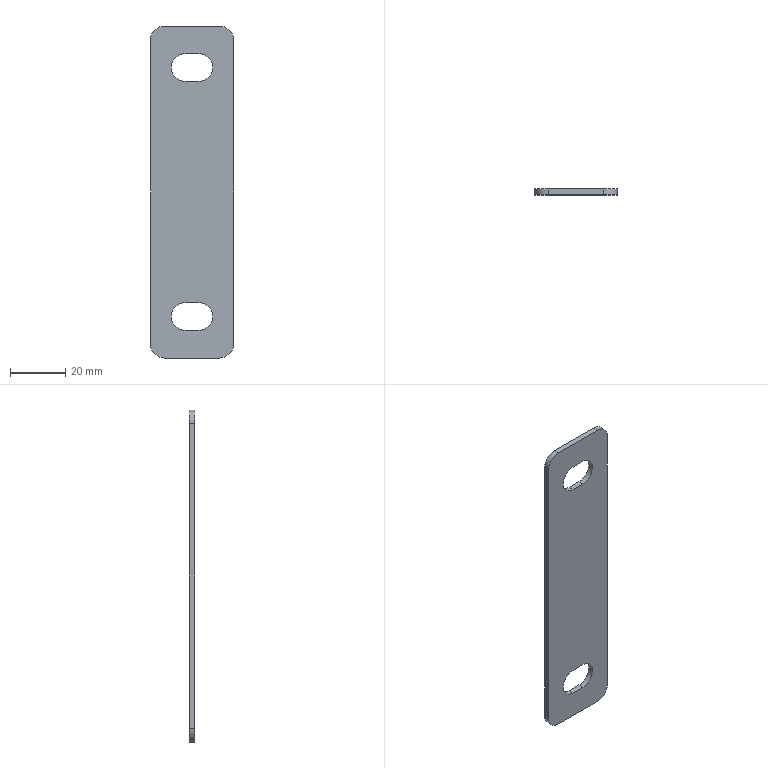Part | SolidWorks | features Fillet 1, FlatPattern 1, ICE 1, SMBaseFlange 1, SheetMetal 1 | 1 solid | 18 faces | box 30 x 2 x 120 mm | volume 6643 mm3 | plane 10 | cylinder 8 | commonest cylinder face diameters 10 x8
STEP:
#1=CARTESIAN_POINT('',(15.,0.,55.));
#2=VERTEX_POINT('',#1);
#3=CARTESIAN_POINT('',(15.,0.,-55.));
#4=VERTEX_POINT('',#3);
#5=CARTESIAN_POINT('',(15.,0.,-60.));
#6=DIRECTION('',(0.,0.,-1.));
#7=VECTOR('',#6,1000.);
#8=LINE('',#5,#7);
#9=EDGE_CURVE('',#2,#4,#8,.T.);
#10=ORIENTED_EDGE('',*,*,#9,.F.);
#11=CARTESIAN_POINT('',(15.,-2.,55.));
#12=VERTEX_POINT('',#11);
#13=CARTESIAN_POINT('',(15.,-2.,55.));
#14=DIRECTION('',(0.,-1.,0.));
#15=VECTOR('',#14,1000.);
#16=LINE('',#13,#15);
#17=EDGE_CURVE('',#2,#12,#16,.T.);
#18=ORIENTED_EDGE('',*,*,#17,.T.);
#19=CARTESIAN_POINT('',(15.,-2.,-55.));
#20=VERTEX_POINT('',#19);
#21=CARTESIAN_POINT('',(15.,-2.,-60.));
#22=DIRECTION('',(0.,0.,-1.));
#23=VECTOR('',#22,1000.);
#24=LINE('',#21,#23);
#25=EDGE_CURVE('',#12,#20,#24,.T.);
#26=ORIENTED_EDGE('',*,*,#25,.T.);
#27=CARTESIAN_POINT('',(15.,-2.,-55.));
#28=DIRECTION('',(0.,1.,0.));
#29=VECTOR('',#28,1000.);
#30=LINE('',#27,#29);
#31=EDGE_CURVE('',#20,#4,#30,.T.);
#32=ORIENTED_EDGE('',*,*,#31,.T.);
#33=EDGE_LOOP('',(#10,#18,#26,#32));
#34=FACE_OUTER_BOUND('',#33,.T.);
#35=CARTESIAN_POINT('',(15.,-2.,-60.));
#36=DIRECTION('',(1.,0.,0.));
#37=DIRECTION('',(0.,0.,-1.));
#38=AXIS2_PLACEMENT_3D('',#35,#36,#37);
#39=PLANE('',#38);
#40=ADVANCED_FACE('',(#34),#39,.T.);
#41=CARTESIAN_POINT('',(-10.,0.,60.));
#42=VERTEX_POINT('',#41);
#43=CARTESIAN_POINT('',(10.,0.,60.));
#44=VERTEX_POINT('',#43);
#45=CARTESIAN_POINT('',(-15.,0.,60.));
#46=DIRECTION('',(1.,0.,0.));
#47=VECTOR('',#46,1000.);
#48=LINE('',#45,#47);
#49=EDGE_CURVE('',#42,#44,#48,.T.);
#50=ORIENTED_EDGE('',*,*,#49,.F.);
#51=CARTESIAN_POINT('',(-10.,-2.,60.));
#52=VERTEX_POINT('',#51);
#53=CARTESIAN_POINT('',(-10.,-2.,60.));
#54=DIRECTION('',(0.,-1.,0.));
#55=VECTOR('',#54,1000.);
#56=LINE('',#53,#55);
#57=EDGE_CURVE('',#42,#52,#56,.T.);
#58=ORIENTED_EDGE('',*,*,#57,.T.);
#59=CARTESIAN_POINT('',(10.,-2.,60.));
#60=VERTEX_POINT('',#59);
#61=CARTESIAN_POINT('',(-15.,-2.,60.));
#62=DIRECTION('',(1.,0.,0.));
#63=VECTOR('',#62,1000.);
#64=LINE('',#61,#63);
#65=EDGE_CURVE('',#52,#60,#64,.T.);
#66=ORIENTED_EDGE('',*,*,#65,.T.);
#67=CARTESIAN_POINT('',(10.,-2.,60.));
#68=DIRECTION('',(0.,1.,0.));
#69=VECTOR('',#68,1000.);
#70=LINE('',#67,#69);
#71=EDGE_CURVE('',#60,#44,#70,.T.);
#72=ORIENTED_EDGE('',*,*,#71,.T.);
#73=EDGE_LOOP('',(#50,#58,#66,#72));
#74=FACE_OUTER_BOUND('',#73,.T.);
#75=CARTESIAN_POINT('',(-15.,-2.,60.));
#76=DIRECTION('',(0.,0.,1.));
#77=DIRECTION('',(1.,0.,0.));
#78=AXIS2_PLACEMENT_3D('',#75,#76,#77);
#79=PLANE('',#78);
#80=ADVANCED_FACE('',(#74),#79,.T.);
#81=CARTESIAN_POINT('',(-15.,-2.,-55.));
#82=VERTEX_POINT('',#81);
#83=CARTESIAN_POINT('',(-15.,-2.,55.));
#84=VERTEX_POINT('',#83);
#85=CARTESIAN_POINT('',(-15.,-2.,-60.));
#86=DIRECTION('',(0.,0.,1.));
#87=VECTOR('',#86,1000.);
#88=LINE('',#85,#87);
#89=EDGE_CURVE('',#82,#84,#88,.T.);
#90=ORIENTED_EDGE('',*,*,#89,.T.);
#91=CARTESIAN_POINT('',(-15.,0.,55.));
#92=VERTEX_POINT('',#91);
#93=CARTESIAN_POINT('',(-15.,-2.,55.));
#94=DIRECTION('',(0.,1.,0.));
#95=VECTOR('',#94,1000.);
#96=LINE('',#93,#95);
#97=EDGE_CURVE('',#84,#92,#96,.T.);
#98=ORIENTED_EDGE('',*,*,#97,.T.);
#99=CARTESIAN_POINT('',(-15.,0.,-55.));
#100=VERTEX_POINT('',#99);
#101=CARTESIAN_POINT('',(-15.,0.,-60.));
#102=DIRECTION('',(0.,0.,1.));
#103=VECTOR('',#102,1000.);
#104=LINE('',#101,#103);
#105=EDGE_CURVE('',#100,#92,#104,.T.);
#106=ORIENTED_EDGE('',*,*,#105,.F.);
#107=CARTESIAN_POINT('',(-15.,-2.,-55.));
#108=DIRECTION('',(0.,-1.,0.));
#109=VECTOR('',#108,1000.);
#110=LINE('',#107,#109);
#111=EDGE_CURVE('',#100,#82,#110,.T.);
#112=ORIENTED_EDGE('',*,*,#111,.T.);
#113=EDGE_LOOP('',(#90,#98,#106,#112));
#114=FACE_OUTER_BOUND('',#113,.T.);
#115=CARTESIAN_POINT('',(-15.,-2.,-60.));
#116=DIRECTION('',(-1.,0.,0.));
#117=DIRECTION('',(0.,0.,1.));
#118=AXIS2_PLACEMENT_3D('',#115,#116,#117);
#119=PLANE('',#118);
#120=ADVANCED_FACE('',(#114),#119,.T.);
#121=CARTESIAN_POINT('',(10.,0.,-60.));
#122=VERTEX_POINT('',#121);
#123=CARTESIAN_POINT('',(-10.,0.,-60.));
#124=VERTEX_POINT('',#123);
#125=CARTESIAN_POINT('',(-15.,0.,-60.));
#126=DIRECTION('',(-1.,0.,0.));
#127=VECTOR('',#126,1000.);
#128=LINE('',#125,#127);
#129=EDGE_CURVE('',#122,#124,#128,.T.);
#130=ORIENTED_EDGE('',*,*,#129,.F.);
#131=CARTESIAN_POINT('',(10.,-2.,-60.));
#132=VERTEX_POINT('',#131);
#133=CARTESIAN_POINT('',(10.,-2.,-60.));
#134=DIRECTION('',(0.,-1.,0.));
#135=VECTOR('',#134,1000.);
#136=LINE('',#133,#135);
#137=EDGE_CURVE('',#122,#132,#136,.T.);
#138=ORIENTED_EDGE('',*,*,#137,.T.);
#139=CARTESIAN_POINT('',(-10.,-2.,-60.));
#140=VERTEX_POINT('',#139);
#141=CARTESIAN_POINT('',(-15.,-2.,-60.));
#142=DIRECTION('',(-1.,0.,0.));
#143=VECTOR('',#142,1000.);
#144=LINE('',#141,#143);
#145=EDGE_CURVE('',#132,#140,#144,.T.);
#146=ORIENTED_EDGE('',*,*,#145,.T.);
#147=CARTESIAN_POINT('',(-10.,-2.,-60.));
#148=DIRECTION('',(0.,1.,0.));
#149=VECTOR('',#148,1000.);
#150=LINE('',#147,#149);
#151=EDGE_CURVE('',#140,#124,#150,.T.);
#152=ORIENTED_EDGE('',*,*,#151,.T.);
#153=EDGE_LOOP('',(#130,#138,#146,#152));
#154=FACE_OUTER_BOUND('',#153,.T.);
#155=CARTESIAN_POINT('',(-15.,-2.,-60.));
#156=DIRECTION('',(0.,0.,-1.));
#157=DIRECTION('',(-1.,0.,0.));
#158=AXIS2_PLACEMENT_3D('',#155,#156,#157);
#159=PLANE('',#158);
#160=ADVANCED_FACE('',(#154),#159,.T.);
#161=CARTESIAN_POINT('',(2.5,-2.,-50.));
#162=VERTEX_POINT('',#161);
#163=CARTESIAN_POINT('',(-2.5,-2.,-50.));
#164=VERTEX_POINT('',#163);
#165=CARTESIAN_POINT('',(0.,-2.,-50.));
#166=DIRECTION('',(-1.,0.,0.));
#167=VECTOR('',#166,1000.);
#168=LINE('',#165,#167);
#169=EDGE_CURVE('',#162,#164,#168,.T.);
#170=ORIENTED_EDGE('',*,*,#169,.T.);
#171=CARTESIAN_POINT('',(-2.5,-2.,-40.));
#172=VERTEX_POINT('',#171);
#173=CARTESIAN_POINT('',(-2.5,-2.,-45.));
#174=DIRECTION('',(0.,1.,0.));
#175=DIRECTION('',(0.,0.,1.));
#176=AXIS2_PLACEMENT_3D('',#173,#174,#175);
#177=CIRCLE('',#176,5.);
#178=EDGE_CURVE('',#164,#172,#177,.T.);
#179=ORIENTED_EDGE('',*,*,#178,.T.);
#180=CARTESIAN_POINT('',(2.5,-2.,-40.));
#181=VERTEX_POINT('',#180);
#182=CARTESIAN_POINT('',(0.,-2.,-40.));
#183=DIRECTION('',(1.,0.,0.));
#184=VECTOR('',#183,1000.);
#185=LINE('',#182,#184);
#186=EDGE_CURVE('',#172,#181,#185,.T.);
#187=ORIENTED_EDGE('',*,*,#186,.T.);
#188=CARTESIAN_POINT('',(2.5,-2.,-45.));
#189=DIRECTION('',(0.,1.,0.));
#190=DIRECTION('',(0.,0.,1.));
#191=AXIS2_PLACEMENT_3D('',#188,#189,#190);
#192=CIRCLE('',#191,5.);
#193=EDGE_CURVE('',#181,#162,#192,.T.);
#194=ORIENTED_EDGE('',*,*,#193,.T.);
#195=EDGE_LOOP('',(#170,#179,#187,#194));
#196=FACE_BOUND('',#195,.T.);
#197=CARTESIAN_POINT('',(2.5,-2.,40.));
#198=VERTEX_POINT('',#197);
#199=CARTESIAN_POINT('',(-2.5,-2.,40.));
#200=VERTEX_POINT('',#199);
#201=CARTESIAN_POINT('',(0.,-2.,40.));
#202=DIRECTION('',(-1.,0.,0.));
#203=VECTOR('',#202,1000.);
#204=LINE('',#201,#203);
#205=EDGE_CURVE('',#198,#200,#204,.T.);
#206=ORIENTED_EDGE('',*,*,#205,.T.);
#207=CARTESIAN_POINT('',(-2.5,-2.,50.));
#208=VERTEX_POINT('',#207);
#209=CARTESIAN_POINT('',(-2.5,-2.,45.));
#210=DIRECTION('',(0.,1.,0.));
#211=DIRECTION('',(0.,0.,1.));
#212=AXIS2_PLACEMENT_3D('',#209,#210,#211);
#213=CIRCLE('',#212,5.);
#214=EDGE_CURVE('',#200,#208,#213,.T.);
#215=ORIENTED_EDGE('',*,*,#214,.T.);
#216=CARTESIAN_POINT('',(2.5,-2.,50.));
#217=VERTEX_POINT('',#216);
#218=CARTESIAN_POINT('',(0.,-2.,50.));
#219=DIRECTION('',(1.,0.,0.));
#220=VECTOR('',#219,1000.);
#221=LINE('',#218,#220);
#222=EDGE_CURVE('',#208,#217,#221,.T.);
#223=ORIENTED_EDGE('',*,*,#222,.T.);
#224=CARTESIAN_POINT('',(2.5,-2.,45.));
#225=DIRECTION('',(0.,1.,0.));
#226=DIRECTION('',(0.,0.,1.));
#227=AXIS2_PLACEMENT_3D('',#224,#225,#226);
#228=CIRCLE('',#227,5.);
#229=EDGE_CURVE('',#217,#198,#228,.T.);
#230=ORIENTED_EDGE('',*,*,#229,.T.);
#231=EDGE_LOOP('',(#206,#215,#223,#230));
#232=FACE_BOUND('',#231,.T.);
#233=ORIENTED_EDGE('',*,*,#65,.F.);
#234=CARTESIAN_POINT('',(-10.,-2.,55.));
#235=DIRECTION('',(0.,-1.,0.));
#236=DIRECTION('',(0.,0.,1.));
#237=AXIS2_PLACEMENT_3D('',#234,#235,#236);
#238=CIRCLE('',#237,5.);
#239=EDGE_CURVE('',#52,#84,#238,.T.);
#240=ORIENTED_EDGE('',*,*,#239,.T.);
#241=ORIENTED_EDGE('',*,*,#89,.F.);
#242=CARTESIAN_POINT('',(-10.,-2.,-55.));
#243=DIRECTION('',(0.,-1.,0.));
#244=DIRECTION('',(0.,0.,1.));
#245=AXIS2_PLACEMENT_3D('',#242,#243,#244);
#246=CIRCLE('',#245,5.);
#247=EDGE_CURVE('',#82,#140,#246,.T.);
#248=ORIENTED_EDGE('',*,*,#247,.T.);
#249=ORIENTED_EDGE('',*,*,#145,.F.);
#250=CARTESIAN_POINT('',(10.,-2.,-55.));
#251=DIRECTION('',(0.,-1.,0.));
#252=DIRECTION('',(0.,0.,1.));
#253=AXIS2_PLACEMENT_3D('',#250,#251,#252);
#254=CIRCLE('',#253,5.);
#255=EDGE_CURVE('',#132,#20,#254,.T.);
#256=ORIENTED_EDGE('',*,*,#255,.T.);
#257=ORIENTED_EDGE('',*,*,#25,.F.);
#258=CARTESIAN_POINT('',(10.,-2.,55.));
#259=DIRECTION('',(0.,-1.,0.));
#260=DIRECTION('',(0.,0.,1.));
#261=AXIS2_PLACEMENT_3D('',#258,#259,#260);
#262=CIRCLE('',#261,5.);
#263=EDGE_CURVE('',#12,#60,#262,.T.);
#264=ORIENTED_EDGE('',*,*,#263,.T.);
#265=EDGE_LOOP('',(#233,#240,#241,#248,#249,#256,#257,#264));
#266=FACE_OUTER_BOUND('',#265,.T.);
#267=CARTESIAN_POINT('',(0.,-2.,0.));
#268=DIRECTION('',(0.,1.,0.));
#269=DIRECTION('',(0.,0.,1.));
#270=AXIS2_PLACEMENT_3D('',#267,#268,#269);
#271=PLANE('',#270);
#272=ADVANCED_FACE('',(#196,#232,#266),#271,.F.);
#273=CARTESIAN_POINT('',(-2.5,0.,-50.));
#274=VERTEX_POINT('',#273);
#275=CARTESIAN_POINT('',(-2.5,0.,-40.));
#276=VERTEX_POINT('',#275);
#277=CARTESIAN_POINT('',(-2.5,0.,-45.));
#278=DIRECTION('',(0.,1.,0.));
#279=DIRECTION('',(0.,0.,1.));
#280=AXIS2_PLACEMENT_3D('',#277,#278,#279);
#281=CIRCLE('',#280,5.);
#282=EDGE_CURVE('',#274,#276,#281,.T.);
#283=ORIENTED_EDGE('',*,*,#282,.F.);
#284=CARTESIAN_POINT('',(2.5,0.,-50.));
#285=VERTEX_POINT('',#284);
#286=CARTESIAN_POINT('',(-2.5,0.,-50.));
#287=DIRECTION('',(-1.,0.,0.));
#288=VECTOR('',#287,1000.);
#289=LINE('',#286,#288);
#290=EDGE_CURVE('',#285,#274,#289,.T.);
#291=ORIENTED_EDGE('',*,*,#290,.F.);
#292=CARTESIAN_POINT('',(2.5,0.,-40.));
#293=VERTEX_POINT('',#292);
#294=CARTESIAN_POINT('',(2.5,0.,-45.));
#295=DIRECTION('',(0.,1.,0.));
#296=DIRECTION('',(0.,0.,1.));
#297=AXIS2_PLACEMENT_3D('',#294,#295,#296);
#298=CIRCLE('',#297,5.);
#299=EDGE_CURVE('',#293,#285,#298,.T.);
#300=ORIENTED_EDGE('',*,*,#299,.F.);
#301=CARTESIAN_POINT('',(-2.5,0.,-40.));
#302=DIRECTION('',(1.,0.,0.));
#303=VECTOR('',#302,1000.);
#304=LINE('',#301,#303);
#305=EDGE_CURVE('',#276,#293,#304,.T.);
#306=ORIENTED_EDGE('',*,*,#305,.F.);
#307=EDGE_LOOP('',(#283,#291,#300,#306));
#308=FACE_BOUND('',#307,.T.);
#309=CARTESIAN_POINT('',(-2.5,0.,40.));
#310=VERTEX_POINT('',#309);
#311=CARTESIAN_POINT('',(-2.5,0.,50.));
#312=VERTEX_POINT('',#311);
#313=CARTESIAN_POINT('',(-2.5,0.,45.));
#314=DIRECTION('',(0.,1.,0.));
#315=DIRECTION('',(0.,0.,-1.));
#316=AXIS2_PLACEMENT_3D('',#313,#314,#315);
#317=CIRCLE('',#316,5.);
#318=EDGE_CURVE('',#310,#312,#317,.T.);
#319=ORIENTED_EDGE('',*,*,#318,.F.);
#320=CARTESIAN_POINT('',(2.5,0.,40.));
#321=VERTEX_POINT('',#320);
#322=CARTESIAN_POINT('',(-2.5,0.,40.));
#323=DIRECTION('',(-1.,0.,0.));
#324=VECTOR('',#323,1000.);
#325=LINE('',#322,#324);
#326=EDGE_CURVE('',#321,#310,#325,.T.);
#327=ORIENTED_EDGE('',*,*,#326,.F.);
#328=CARTESIAN_POINT('',(2.5,0.,50.));
#329=VERTEX_POINT('',#328);
#330=CARTESIAN_POINT('',(2.5,0.,45.));
#331=DIRECTION('',(0.,1.,0.));
#332=DIRECTION('',(0.,0.,-1.));
#333=AXIS2_PLACEMENT_3D('',#330,#331,#332);
#334=CIRCLE('',#333,5.);
#335=EDGE_CURVE('',#329,#321,#334,.T.);
#336=ORIENTED_EDGE('',*,*,#335,.F.);
#337=CARTESIAN_POINT('',(-2.5,0.,50.));
#338=DIRECTION('',(1.,0.,0.));
#339=VECTOR('',#338,1000.);
#340=LINE('',#337,#339);
#341=EDGE_CURVE('',#312,#329,#340,.T.);
#342=ORIENTED_EDGE('',*,*,#341,.F.);
#343=EDGE_LOOP('',(#319,#327,#336,#342));
#344=FACE_BOUND('',#343,.T.);
#345=ORIENTED_EDGE('',*,*,#105,.T.);
#346=CARTESIAN_POINT('',(-10.,0.,55.));
#347=DIRECTION('',(0.,1.,0.));
#348=DIRECTION('',(0.,0.,1.));
#349=AXIS2_PLACEMENT_3D('',#346,#347,#348);
#350=CIRCLE('',#349,5.);
#351=EDGE_CURVE('',#92,#42,#350,.T.);
#352=ORIENTED_EDGE('',*,*,#351,.T.);
#353=ORIENTED_EDGE('',*,*,#49,.T.);
#354=CARTESIAN_POINT('',(10.,0.,55.));
#355=DIRECTION('',(0.,1.,0.));
#356=DIRECTION('',(0.,0.,1.));
#357=AXIS2_PLACEMENT_3D('',#354,#355,#356);
#358=CIRCLE('',#357,5.);
#359=EDGE_CURVE('',#44,#2,#358,.T.);
#360=ORIENTED_EDGE('',*,*,#359,.T.);
#361=ORIENTED_EDGE('',*,*,#9,.T.);
#362=CARTESIAN_POINT('',(10.,0.,-55.));
#363=DIRECTION('',(0.,1.,0.));
#364=DIRECTION('',(0.,0.,1.));
#365=AXIS2_PLACEMENT_3D('',#362,#363,#364);
#366=CIRCLE('',#365,5.);
#367=EDGE_CURVE('',#4,#122,#366,.T.);
#368=ORIENTED_EDGE('',*,*,#367,.T.);
#369=ORIENTED_EDGE('',*,*,#129,.T.);
#370=CARTESIAN_POINT('',(-10.,0.,-55.));
#371=DIRECTION('',(0.,1.,0.));
#372=DIRECTION('',(0.,0.,1.));
#373=AXIS2_PLACEMENT_3D('',#370,#371,#372);
#374=CIRCLE('',#373,5.);
#375=EDGE_CURVE('',#124,#100,#374,.T.);
#376=ORIENTED_EDGE('',*,*,#375,.T.);
#377=EDGE_LOOP('',(#345,#352,#353,#360,#361,#368,#369,#376));
#378=FACE_OUTER_BOUND('',#377,.T.);
#379=CARTESIAN_POINT('',(0.,0.,0.));
#380=DIRECTION('',(0.,1.,0.));
#381=DIRECTION('',(0.,0.,1.));
#382=AXIS2_PLACEMENT_3D('',#379,#380,#381);
#383=PLANE('',#382);
#384=ADVANCED_FACE('',(#308,#344,#378),#383,.T.);
#385=CARTESIAN_POINT('',(-2.5,-10.,40.));
#386=DIRECTION('',(0.,1.,0.));
#387=VECTOR('',#386,1000.);
#388=LINE('',#385,#387);
#389=EDGE_CURVE('',#200,#310,#388,.T.);
#390=ORIENTED_EDGE('',*,*,#389,.T.);
#391=ORIENTED_EDGE('',*,*,#318,.T.);
#392=CARTESIAN_POINT('',(-2.5,-10.,50.));
#393=DIRECTION('',(0.,1.,0.));
#394=VECTOR('',#393,1000.);
#395=LINE('',#392,#394);
#396=EDGE_CURVE('',#208,#312,#395,.T.);
#397=ORIENTED_EDGE('',*,*,#396,.F.);
#398=ORIENTED_EDGE('',*,*,#214,.F.);
#399=EDGE_LOOP('',(#390,#391,#397,#398));
#400=FACE_OUTER_BOUND('',#399,.T.);
#401=CARTESIAN_POINT('',(-2.5,-10.,45.));
#402=DIRECTION('',(0.,1.,0.));
#403=DIRECTION('',(0.,0.,1.));
#404=AXIS2_PLACEMENT_3D('',#401,#402,#403);
#405=CYLINDRICAL_SURFACE('',#404,5.);
#406=ADVANCED_FACE('',(#400),#405,.F.);
#407=CARTESIAN_POINT('',(2.5,-10.,40.));
#408=DIRECTION('',(0.,1.,0.));
#409=VECTOR('',#408,1000.);
#410=LINE('',#407,#409);
#411=EDGE_CURVE('',#198,#321,#410,.T.);
#412=ORIENTED_EDGE('',*,*,#411,.T.);
#413=ORIENTED_EDGE('',*,*,#326,.T.);
#414=ORIENTED_EDGE('',*,*,#389,.F.);
#415=ORIENTED_EDGE('',*,*,#205,.F.);
#416=EDGE_LOOP('',(#412,#413,#414,#415));
#417=FACE_OUTER_BOUND('',#416,.T.);
#418=CARTESIAN_POINT('',(-2.5,-10.,40.));
#419=DIRECTION('',(0.,0.,-1.));
#420=DIRECTION('',(-1.,0.,0.));
#421=AXIS2_PLACEMENT_3D('',#418,#419,#420);
#422=PLANE('',#421);
#423=ADVANCED_FACE('',(#417),#422,.F.);
#424=CARTESIAN_POINT('',(2.5,-10.,50.));
#425=DIRECTION('',(0.,1.,0.));
#426=VECTOR('',#425,1000.);
#427=LINE('',#424,#426);
#428=EDGE_CURVE('',#217,#329,#427,.T.);
#429=ORIENTED_EDGE('',*,*,#428,.T.);
#430=ORIENTED_EDGE('',*,*,#335,.T.);
#431=ORIENTED_EDGE('',*,*,#411,.F.);
#432=ORIENTED_EDGE('',*,*,#229,.F.);
#433=EDGE_LOOP('',(#429,#430,#431,#432));
#434=FACE_OUTER_BOUND('',#433,.T.);
#435=CARTESIAN_POINT('',(2.5,-10.,45.));
#436=DIRECTION('',(0.,1.,0.));
#437=DIRECTION('',(0.,0.,1.));
#438=AXIS2_PLACEMENT_3D('',#435,#436,#437);
#439=CYLINDRICAL_SURFACE('',#438,5.);
#440=ADVANCED_FACE('',(#434),#439,.F.);
#441=ORIENTED_EDGE('',*,*,#396,.T.);
#442=ORIENTED_EDGE('',*,*,#341,.T.);
#443=ORIENTED_EDGE('',*,*,#428,.F.);
#444=ORIENTED_EDGE('',*,*,#222,.F.);
#445=EDGE_LOOP('',(#441,#442,#443,#444));
#446=FACE_OUTER_BOUND('',#445,.T.);
#447=CARTESIAN_POINT('',(-2.5,-10.,50.));
#448=DIRECTION('',(0.,0.,1.));
#449=DIRECTION('',(1.,0.,0.));
#450=AXIS2_PLACEMENT_3D('',#447,#448,#449);
#451=PLANE('',#450);
#452=ADVANCED_FACE('',(#446),#451,.F.);
#453=CARTESIAN_POINT('',(-2.5,-10.,-50.));
#454=DIRECTION('',(0.,1.,0.));
#455=VECTOR('',#454,1000.);
#456=LINE('',#453,#455);
#457=EDGE_CURVE('',#164,#274,#456,.T.);
#458=ORIENTED_EDGE('',*,*,#457,.T.);
#459=ORIENTED_EDGE('',*,*,#282,.T.);
#460=CARTESIAN_POINT('',(-2.5,-10.,-40.));
#461=DIRECTION('',(0.,1.,0.));
#462=VECTOR('',#461,1000.);
#463=LINE('',#460,#462);
#464=EDGE_CURVE('',#172,#276,#463,.T.);
#465=ORIENTED_EDGE('',*,*,#464,.F.);
#466=ORIENTED_EDGE('',*,*,#178,.F.);
#467=EDGE_LOOP('',(#458,#459,#465,#466));
#468=FACE_OUTER_BOUND('',#467,.T.);
#469=CARTESIAN_POINT('',(-2.5,-10.,-45.));
#470=DIRECTION('',(0.,1.,0.));
#471=DIRECTION('',(0.,0.,1.));
#472=AXIS2_PLACEMENT_3D('',#469,#470,#471);
#473=CYLINDRICAL_SURFACE('',#472,5.);
#474=ADVANCED_FACE('',(#468),#473,.F.);
#475=CARTESIAN_POINT('',(2.5,-10.,-50.));
#476=DIRECTION('',(0.,1.,0.));
#477=VECTOR('',#476,1000.);
#478=LINE('',#475,#477);
#479=EDGE_CURVE('',#162,#285,#478,.T.);
#480=ORIENTED_EDGE('',*,*,#479,.T.);
#481=ORIENTED_EDGE('',*,*,#290,.T.);
#482=ORIENTED_EDGE('',*,*,#457,.F.);
#483=ORIENTED_EDGE('',*,*,#169,.F.);
#484=EDGE_LOOP('',(#480,#481,#482,#483));
#485=FACE_OUTER_BOUND('',#484,.T.);
#486=CARTESIAN_POINT('',(-2.5,-10.,-50.));
#487=DIRECTION('',(0.,0.,-1.));
#488=DIRECTION('',(-1.,0.,0.));
#489=AXIS2_PLACEMENT_3D('',#486,#487,#488);
#490=PLANE('',#489);
#491=ADVANCED_FACE('',(#485),#490,.F.);
#492=CARTESIAN_POINT('',(2.5,-10.,-40.));
#493=DIRECTION('',(0.,1.,0.));
#494=VECTOR('',#493,1000.);
#495=LINE('',#492,#494);
#496=EDGE_CURVE('',#181,#293,#495,.T.);
#497=ORIENTED_EDGE('',*,*,#496,.T.);
#498=ORIENTED_EDGE('',*,*,#299,.T.);
#499=ORIENTED_EDGE('',*,*,#479,.F.);
#500=ORIENTED_EDGE('',*,*,#193,.F.);
#501=EDGE_LOOP('',(#497,#498,#499,#500));
#502=FACE_OUTER_BOUND('',#501,.T.);
#503=CARTESIAN_POINT('',(2.5,-10.,-45.));
#504=DIRECTION('',(0.,1.,0.));
#505=DIRECTION('',(0.,0.,1.));
#506=AXIS2_PLACEMENT_3D('',#503,#504,#505);
#507=CYLINDRICAL_SURFACE('',#506,5.);
#508=ADVANCED_FACE('',(#502),#507,.F.);
#509=ORIENTED_EDGE('',*,*,#464,.T.);
#510=ORIENTED_EDGE('',*,*,#305,.T.);
#511=ORIENTED_EDGE('',*,*,#496,.F.);
#512=ORIENTED_EDGE('',*,*,#186,.F.);
#513=EDGE_LOOP('',(#509,#510,#511,#512));
#514=FACE_OUTER_BOUND('',#513,.T.);
#515=CARTESIAN_POINT('',(-2.5,-10.,-40.));
#516=DIRECTION('',(0.,0.,1.));
#517=DIRECTION('',(1.,0.,0.));
#518=AXIS2_PLACEMENT_3D('',#515,#516,#517);
#519=PLANE('',#518);
#520=ADVANCED_FACE('',(#514),#519,.F.);
#521=ORIENTED_EDGE('',*,*,#239,.F.);
#522=ORIENTED_EDGE('',*,*,#57,.F.);
#523=ORIENTED_EDGE('',*,*,#351,.F.);
#524=ORIENTED_EDGE('',*,*,#97,.F.);
#525=EDGE_LOOP('',(#521,#522,#523,#524));
#526=FACE_OUTER_BOUND('',#525,.T.);
#527=CARTESIAN_POINT('',(-10.,-2.,55.));
#528=DIRECTION('',(0.,1.,0.));
#529=DIRECTION('',(0.,0.,1.));
#530=AXIS2_PLACEMENT_3D('',#527,#528,#529);
#531=CYLINDRICAL_SURFACE('',#530,5.);
#532=ADVANCED_FACE('',(#526),#531,.T.);
#533=ORIENTED_EDGE('',*,*,#263,.F.);
#534=ORIENTED_EDGE('',*,*,#17,.F.);
#535=ORIENTED_EDGE('',*,*,#359,.F.);
#536=ORIENTED_EDGE('',*,*,#71,.F.);
#537=EDGE_LOOP('',(#533,#534,#535,#536));
#538=FACE_OUTER_BOUND('',#537,.T.);
#539=CARTESIAN_POINT('',(10.,-2.,55.));
#540=DIRECTION('',(0.,1.,0.));
#541=DIRECTION('',(0.,0.,1.));
#542=AXIS2_PLACEMENT_3D('',#539,#540,#541);
#543=CYLINDRICAL_SURFACE('',#542,5.);
#544=ADVANCED_FACE('',(#538),#543,.T.);
#545=ORIENTED_EDGE('',*,*,#255,.F.);
#546=ORIENTED_EDGE('',*,*,#137,.F.);
#547=ORIENTED_EDGE('',*,*,#367,.F.);
#548=ORIENTED_EDGE('',*,*,#31,.F.);
#549=EDGE_LOOP('',(#545,#546,#547,#548));
#550=FACE_OUTER_BOUND('',#549,.T.);
#551=CARTESIAN_POINT('',(10.,-2.,-55.));
#552=DIRECTION('',(0.,1.,0.));
#553=DIRECTION('',(0.,0.,1.));
#554=AXIS2_PLACEMENT_3D('',#551,#552,#553);
#555=CYLINDRICAL_SURFACE('',#554,5.);
#556=ADVANCED_FACE('',(#550),#555,.T.);
#557=ORIENTED_EDGE('',*,*,#247,.F.);
#558=ORIENTED_EDGE('',*,*,#111,.F.);
#559=ORIENTED_EDGE('',*,*,#375,.F.);
#560=ORIENTED_EDGE('',*,*,#151,.F.);
#561=EDGE_LOOP('',(#557,#558,#559,#560));
#562=FACE_OUTER_BOUND('',#561,.T.);
#563=CARTESIAN_POINT('',(-10.,-2.,-55.));
#564=DIRECTION('',(0.,1.,0.));
#565=DIRECTION('',(0.,0.,1.));
#566=AXIS2_PLACEMENT_3D('',#563,#564,#565);
#567=CYLINDRICAL_SURFACE('',#566,5.);
#568=ADVANCED_FACE('',(#562),#567,.T.);
#569=CLOSED_SHELL('',(#40,#80,#120,#160,#272,#384,#406,#423,#440,#452,#474,#491,#508,#520,#532,#544,#556,#568));
#570=MANIFOLD_SOLID_BREP('',#569);
#571=CARTESIAN_POINT('',(0.,0.,0.));
#572=DIRECTION('',(0.,0.,1.));
#573=DIRECTION('',(1.,0.,0.));
#574=AXIS2_PLACEMENT_3D('',#571,#572,#573);
#575=(LENGTH_UNIT()NAMED_UNIT(*)SI_UNIT(.MILLI.,.METRE.));
#576=UNCERTAINTY_MEASURE_WITH_UNIT(LENGTH_MEASURE(0.00001),#575,'','');
#577=(NAMED_UNIT(*)PLANE_ANGLE_UNIT()SI_UNIT($,.RADIAN.));
#578=(NAMED_UNIT(*)SI_UNIT($,.STERADIAN.)SOLID_ANGLE_UNIT());
#579=(GEOMETRIC_REPRESENTATION_CONTEXT(3)GLOBAL_UNCERTAINTY_ASSIGNED_CONTEXT((#576))GLOBAL_UNIT_ASSIGNED_CONTEXT((#575,#577,#578))REPRESENTATION_CONTEXT('',''));
#580=ADVANCED_BREP_SHAPE_REPRESENTATION('',(#570,#574),#579);